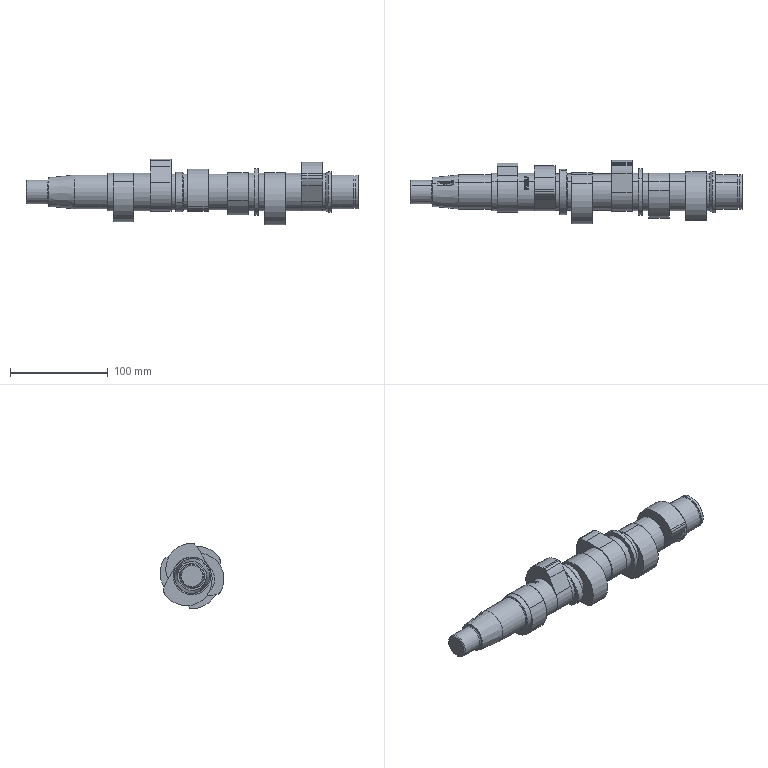Part | SolidWorks | features BaseBody 1 | 1 solid | 247 faces | box 340 x 65.54 x 67 mm | volume 445477 mm3 | plane 88 | cylinder 81 | spline 60 | torus 12 | cone 6 | commonest cylinder face diameters 38.5 x17 39 x9 53 x8 8 x7 35 x6 37 x6